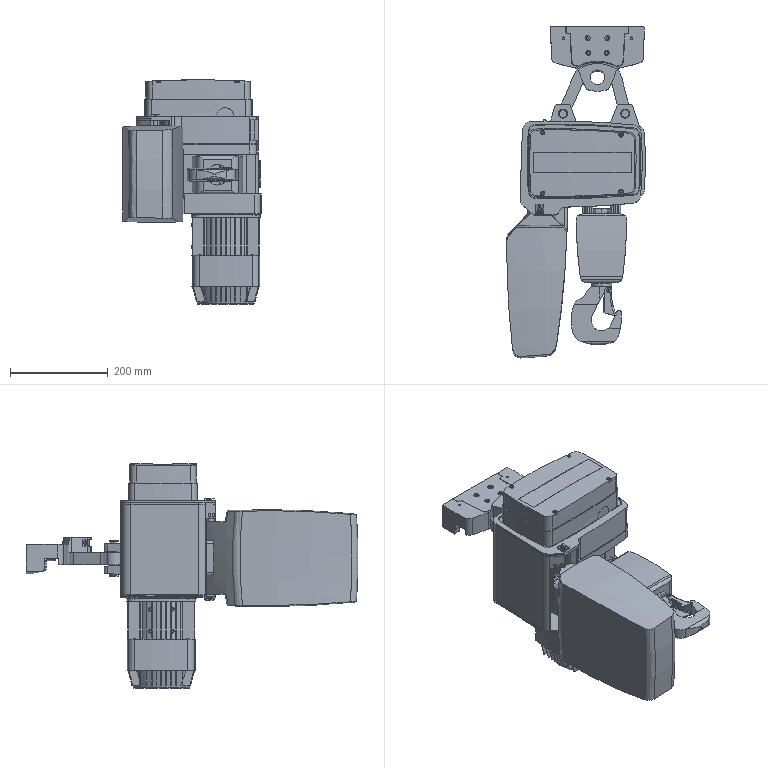Part | SolidWorks | features BaseBody 17, ICE 1, Scale 1 | 17 solids | 1986 faces | box 284.321 x 680.473 x 459.6 mm | volume 19540266 mm3 | plane 1027 | cylinder 661 | torus 156 | cone 138 | sphere 4 | commonest cylinder face diameters 7.5 x60 4.5 x35 117.75 x32 9 x27 12 x27 6.75 x24